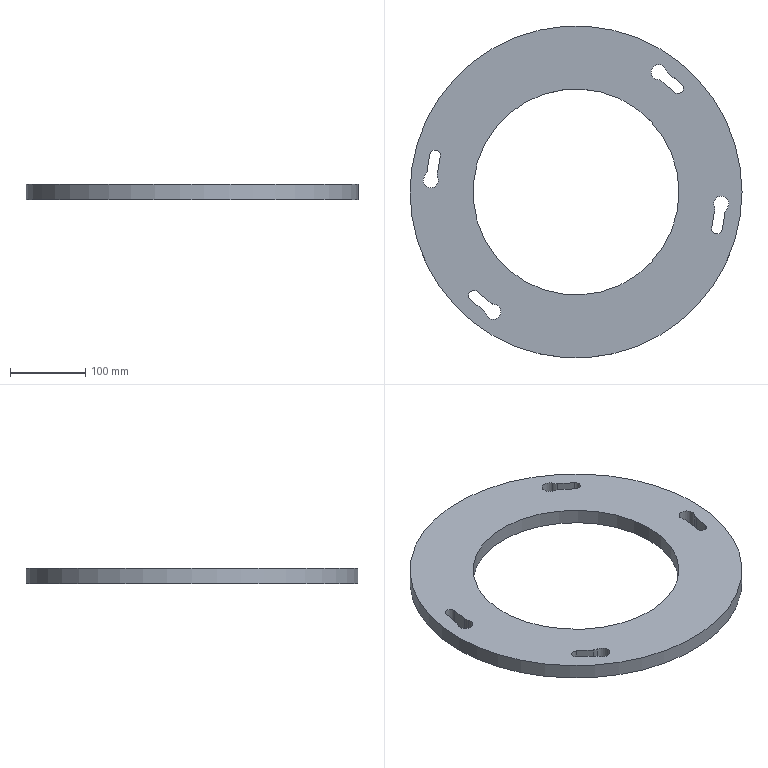NC program | NX | posted with a generic post | part box 440 x 440 x 20 mm
Lines 1 to 784 of 7039:
N10 G17 G21 G94 G90
(ZLEVEL_PROFILE_COPY_1 , TOOL : D10)
N12 T10 M6
N14 G54
N16 G17 G0 G90 X-122.22 Y-146.019 S2200 M3
N18 G43 Z80. H10
N20 Z1.5
N22 G94 G1 X-134.503 Y-135.858 Z0.665 F2200.
N24 X-134.722 Y-135.75 Z0.652
N26 X-135.025 Y-135.606 Z0.634
N28 X-135.519 Y-135.541 Z0.608
N30 X-136.012 Y-135.608 Z0.582
N32 X-136.314 Y-135.752 Z0.564
N34 Y-135.831 Z0.56
N36 X-136.345 Y-135.857 Z0.558
N38 X-136.423 Y-135.84 Z0.554
N40 X-136.449 Y-135.824 Z0.552
N42 X-136.738 Y-135.992 Z0.535
N44 X-137.073 Y-136.368 Z0.509
N46 X-137.215 Y-136.689 Z0.49
N48 X-137.347 Y-136.996 Z0.473
N50 X-137.354 Y-137.814 Z0.43
N52 X-137.214 Y-138.155 Z0.41
N54 X-137.081 Y-138.462 Z0.393
N56 X-136.953 Y-138.633 Z0.382
N58 X-128.11 Y-145.949 Z-0.22
N60 X-119.524 Y-153.051
N62 G2 X-114.128 Y-160.588 R18.15
N64 G3 X-112.621 Y-162.654 R4.85
N66 G1 X-112.486 Y-162.758
N68 G3 X-106.443 Y-162.552 R4.85
N70 G1 X-105.654 Y-161.694
N72 G3 X-104.895 Y-160.066 R4.85
N74 G1 X-104.918 Y-160.045
N76 X-104.885 Y-160.028
N78 G3 X-104.883 Y-157.71 R4.85
N80 G1 X-104.918 Y-157.689
N82 X-104.893 Y-157.672
N84 G3 X-105.845 Y-155.789 R4.85
N86 G1 X-106.646 Y-155.014
N88 G3 X-108.751 Y-154.089 R4.85
N90 G2 X-117.166 Y-150.2 R18.15
N92 G1 X-134.336 Y-135.996
N94 G3 X-136.314 Y-135.752 R1.85
N96 G1 X-136.305 Y-135.819
N98 X-136.359 Y-135.863
N100 X-136.423 Y-135.84
N102 X-136.449 Y-135.824
N104 G3 X-136.695 Y-138.846 R1.85
N106 G1 X-128.11 Y-145.949
N108 X-119.549 Y-153.03 Z-0.414
N110 X-119.266 Y-153.269 Z-0.42
N112 X-118.988 Y-153.513 Z-0.427
N114 X-118.714 Y-153.763 Z-0.433
N116 X-118.446 Y-154.018 Z-0.44
N118 G2 X-114.128 Y-160.588 R18.15
N120 G3 X-112.621 Y-162.654 R4.85
N122 G1 X-112.486 Y-162.758
N124 G3 X-106.443 Y-162.552 R4.85
N126 G1 X-105.654 Y-161.694
N128 G3 X-104.895 Y-160.066 R4.85
N130 G1 X-104.918 Y-160.045
N132 X-104.885 Y-160.028
N134 G3 X-104.883 Y-157.71 R4.85
N136 G1 X-104.918 Y-157.689
N138 X-104.893 Y-157.672
N140 G3 X-105.845 Y-155.789 R4.85
N142 G1 X-106.646 Y-155.014
N144 G3 X-108.751 Y-154.089 R4.85
N146 G2 X-117.166 Y-150.2 R18.15
N148 G1 X-134.336 Y-135.996
N150 G3 X-136.314 Y-135.752 R1.85
N152 G1 X-136.305 Y-135.819
N154 X-136.359 Y-135.863
N156 X-136.423 Y-135.84
N158 X-136.449 Y-135.824
N160 G3 X-136.695 Y-138.846 R1.85
N162 G1 X-128.11 Y-145.949
N164 X-119.549 Y-153.03 Z-0.633
N166 X-119.266 Y-153.269 Z-0.64
N168 X-118.988 Y-153.513 Z-0.646
N170 X-118.714 Y-153.763 Z-0.653
N172 X-118.446 Y-154.018 Z-0.659
N174 G2 X-114.128 Y-160.588 R18.15
N176 G3 X-112.621 Y-162.654 R4.85
N178 G1 X-112.486 Y-162.758
N180 G3 X-106.443 Y-162.552 R4.85
N182 G1 X-105.654 Y-161.694
N184 G3 X-104.895 Y-160.066 R4.85
N186 G1 X-104.918 Y-160.045
N188 X-104.885 Y-160.028
N190 G3 X-104.883 Y-157.71 R4.85
N192 G1 X-104.918 Y-157.689
N194 X-104.893 Y-157.672
N196 G3 X-105.845 Y-155.789 R4.85
N198 G1 X-106.646 Y-155.014
N200 G3 X-108.751 Y-154.089 R4.85
N202 G2 X-117.166 Y-150.2 R18.15
N204 G1 X-134.336 Y-135.996
N206 G3 X-136.314 Y-135.752 R1.85
N208 G1 X-136.305 Y-135.819
N210 X-136.359 Y-135.863
N212 X-136.423 Y-135.84
N214 X-136.449 Y-135.824
N216 G3 X-136.695 Y-138.846 R1.85
N218 G1 X-128.11 Y-145.949
N220 X-119.549 Y-153.03 Z-0.853
N222 X-119.266 Y-153.269 Z-0.86
N224 X-118.988 Y-153.513 Z-0.866
N226 X-118.714 Y-153.763 Z-0.873
N228 X-118.446 Y-154.018 Z-0.879
N230 G2 X-114.128 Y-160.588 R18.15
N232 G3 X-112.621 Y-162.654 R4.85
N234 G1 X-112.486 Y-162.758
N236 G3 X-106.443 Y-162.552 R4.85
N238 G1 X-105.654 Y-161.694
N240 G3 X-104.895 Y-160.066 R4.85
N242 G1 X-104.918 Y-160.045
N244 X-104.885 Y-160.028
N246 G3 X-104.883 Y-157.71 R4.85
N248 G1 X-104.918 Y-157.689
N250 X-104.893 Y-157.672
N252 G3 X-105.845 Y-155.789 R4.85
N254 G1 X-106.646 Y-155.014
N256 G3 X-108.751 Y-154.089 R4.85
N258 G2 X-117.166 Y-150.2 R18.15
N260 G1 X-134.336 Y-135.996
N262 G3 X-136.314 Y-135.752 R1.85
N264 G1 X-136.305 Y-135.819
N266 X-136.359 Y-135.863
N268 X-136.423 Y-135.84
N270 X-136.449 Y-135.824
N272 G3 X-136.695 Y-138.846 R1.85
N274 G1 X-128.11 Y-145.949
N276 X-119.549 Y-153.03 Z-1.073
N278 X-119.266 Y-153.269 Z-1.08
N280 X-118.988 Y-153.513 Z-1.086
N282 X-118.714 Y-153.763 Z-1.092
N284 X-118.446 Y-154.018 Z-1.099
N286 G2 X-114.128 Y-160.588 R18.15
N288 G3 X-112.621 Y-162.654 R4.85
N290 G1 X-112.486 Y-162.758
N292 G3 X-106.443 Y-162.552 R4.85
N294 G1 X-105.654 Y-161.694
N296 G3 X-104.895 Y-160.066 R4.85
N298 G1 X-104.918 Y-160.045
N300 X-104.885 Y-160.028
N302 G3 X-104.883 Y-157.71 R4.85
N304 G1 X-104.918 Y-157.689
N306 X-104.893 Y-157.672
N308 G3 X-105.845 Y-155.789 R4.85
N310 G1 X-106.646 Y-155.014
N312 G3 X-108.751 Y-154.089 R4.85
N314 G2 X-117.166 Y-150.2 R18.15
N316 G1 X-134.336 Y-135.996
N318 G3 X-136.314 Y-135.752 R1.85
N320 G1 X-136.305 Y-135.819
N322 X-136.359 Y-135.863
N324 X-136.423 Y-135.84
N326 X-136.449 Y-135.824
N328 G3 X-136.695 Y-138.846 R1.85
N330 G1 X-128.11 Y-145.949
N332 X-119.549 Y-153.03 Z-1.293
N334 X-119.266 Y-153.269 Z-1.299
N336 X-118.988 Y-153.513 Z-1.306
N338 X-118.714 Y-153.763 Z-1.312
N340 X-118.446 Y-154.018 Z-1.319
N342 G2 X-114.128 Y-160.588 R18.15
N344 G3 X-112.621 Y-162.654 R4.85
N346 G1 X-112.486 Y-162.758
N348 G3 X-106.443 Y-162.552 R4.85
N350 G1 X-105.654 Y-161.694
N352 G3 X-104.895 Y-160.066 R4.85
N354 G1 X-104.918 Y-160.045
N356 X-104.885 Y-160.028
N358 G3 X-104.883 Y-157.71 R4.85
N360 G1 X-104.918 Y-157.689
N362 X-104.893 Y-157.672
N364 G3 X-105.845 Y-155.789 R4.85
N366 G1 X-106.646 Y-155.014
N368 G3 X-108.751 Y-154.089 R4.85
N370 G2 X-117.166 Y-150.2 R18.15
N372 G1 X-134.336 Y-135.996
N374 G3 X-136.314 Y-135.752 R1.85
N376 G1 X-136.305 Y-135.819
N378 X-136.359 Y-135.863
N380 X-136.423 Y-135.84
N382 X-136.449 Y-135.824
N384 G3 X-136.695 Y-138.846 R1.85
N386 G1 X-128.11 Y-145.949
N388 X-119.549 Y-153.03 Z-1.513
N390 X-119.266 Y-153.269 Z-1.519
N392 X-118.988 Y-153.513 Z-1.526
N394 X-118.714 Y-153.763 Z-1.532
N396 X-118.446 Y-154.018 Z-1.538
N398 G2 X-114.128 Y-160.588 R18.15
N400 G3 X-112.621 Y-162.654 R4.85
N402 G1 X-112.486 Y-162.758
N404 G3 X-106.443 Y-162.552 R4.85
N406 G1 X-105.654 Y-161.694
N408 G3 X-104.895 Y-160.066 R4.85
N410 G1 X-104.918 Y-160.045
N412 X-104.885 Y-160.028
N414 G3 X-104.883 Y-157.71 R4.85
N416 G1 X-104.918 Y-157.689
N418 X-104.893 Y-157.672
N420 G3 X-105.845 Y-155.789 R4.85
N422 G1 X-106.646 Y-155.014
N424 G3 X-108.751 Y-154.089 R4.85
N426 G2 X-117.166 Y-150.2 R18.15
N428 G1 X-134.336 Y-135.996
N430 G3 X-136.314 Y-135.752 R1.85
N432 G1 X-136.305 Y-135.819
N434 X-136.359 Y-135.863
N436 X-136.423 Y-135.84
N438 X-136.449 Y-135.824
N440 G3 X-136.695 Y-138.846 R1.85
N442 G1 X-128.11 Y-145.949
N444 X-119.549 Y-153.03 Z-1.732
N446 X-119.266 Y-153.269 Z-1.739
N448 X-118.988 Y-153.513 Z-1.745
N450 X-118.714 Y-153.763 Z-1.752
N452 X-118.446 Y-154.018 Z-1.758
N454 G2 X-114.128 Y-160.588 R18.15
N456 G3 X-112.621 Y-162.654 R4.85
N458 G1 X-112.486 Y-162.758
N460 G3 X-106.443 Y-162.552 R4.85
N462 G1 X-105.654 Y-161.694
N464 G3 X-104.895 Y-160.066 R4.85
N466 G1 X-104.918 Y-160.045
N468 X-104.885 Y-160.028
N470 G3 X-104.883 Y-157.71 R4.85
N472 G1 X-104.918 Y-157.689
N474 X-104.893 Y-157.672
N476 G3 X-105.845 Y-155.789 R4.85
N478 G1 X-106.646 Y-155.014
N480 G3 X-108.751 Y-154.089 R4.85
N482 G2 X-117.166 Y-150.2 R18.15
N484 G1 X-134.336 Y-135.996
N486 G3 X-136.314 Y-135.752 R1.85
N488 G1 X-136.305 Y-135.819
N490 X-136.359 Y-135.863
N492 X-136.423 Y-135.84
N494 X-136.449 Y-135.824
N496 G3 X-136.695 Y-138.846 R1.85
N498 G1 X-128.11 Y-145.949
N500 X-119.549 Y-153.03 Z-1.952
N502 X-119.266 Y-153.269 Z-1.959
N504 X-118.988 Y-153.513 Z-1.965
N506 X-118.714 Y-153.763 Z-1.972
N508 X-118.446 Y-154.018 Z-1.978
N510 G2 X-114.128 Y-160.588 R18.15
N512 G3 X-112.621 Y-162.654 R4.85
N514 G1 X-112.486 Y-162.758
N516 G3 X-106.443 Y-162.552 R4.85
N518 G1 X-105.654 Y-161.694
N520 G3 X-104.895 Y-160.066 R4.85
N522 G1 X-104.918 Y-160.045
N524 X-104.885 Y-160.028
N526 G3 X-104.883 Y-157.71 R4.85
N528 G1 X-104.918 Y-157.689
N530 X-104.893 Y-157.672
N532 G3 X-105.845 Y-155.789 R4.85
N534 G1 X-106.646 Y-155.014
N536 G3 X-108.751 Y-154.089 R4.85
N538 G2 X-117.166 Y-150.2 R18.15
N540 G1 X-134.336 Y-135.996
N542 G3 X-136.314 Y-135.752 R1.85
N544 G1 X-136.305 Y-135.819
N546 X-136.359 Y-135.863
N548 X-136.423 Y-135.84
N550 X-136.449 Y-135.824
N552 G3 X-136.695 Y-138.846 R1.85
N554 G1 X-128.11 Y-145.949
N556 X-119.549 Y-153.03 Z-2.172
N558 X-119.266 Y-153.269 Z-2.178
N560 X-118.988 Y-153.513 Z-2.185
N562 X-118.714 Y-153.763 Z-2.191
N564 X-118.446 Y-154.018 Z-2.198
N566 G2 X-114.128 Y-160.588 R18.15
N568 G3 X-112.621 Y-162.654 R4.85
N570 G1 X-112.486 Y-162.758
N572 G3 X-106.443 Y-162.552 R4.85
N574 G1 X-105.654 Y-161.694
N576 G3 X-104.895 Y-160.066 R4.85
N578 G1 X-104.918 Y-160.045
N580 X-104.885 Y-160.028
N582 G3 X-104.883 Y-157.71 R4.85
N584 G1 X-104.918 Y-157.689
N586 X-104.893 Y-157.672
N588 G3 X-105.845 Y-155.789 R4.85
N590 G1 X-106.646 Y-155.014
N592 G3 X-108.751 Y-154.089 R4.85
N594 G2 X-117.166 Y-150.2 R18.15
N596 G1 X-134.336 Y-135.996
N598 G3 X-136.314 Y-135.752 R1.85
N600 G1 X-136.305 Y-135.819
N602 X-136.359 Y-135.863
N604 X-136.423 Y-135.84
N606 X-136.449 Y-135.824
N608 G3 X-136.695 Y-138.846 R1.85
N610 G1 X-128.11 Y-145.949
N612 X-119.549 Y-153.03 Z-2.392
N614 X-119.266 Y-153.269 Z-2.398
N616 X-118.988 Y-153.513 Z-2.405
N618 X-118.714 Y-153.763 Z-2.411
N620 X-118.446 Y-154.018 Z-2.418
N622 G2 X-114.128 Y-160.588 R18.15
N624 G3 X-112.621 Y-162.654 R4.85
N626 G1 X-112.486 Y-162.758
N628 G3 X-106.443 Y-162.552 R4.85
N630 G1 X-105.654 Y-161.694
N632 G3 X-104.895 Y-160.066 R4.85
N634 G1 X-104.918 Y-160.045
N636 X-104.885 Y-160.028
N638 G3 X-104.883 Y-157.71 R4.85
N640 G1 X-104.918 Y-157.689
N642 X-104.893 Y-157.672
N644 G3 X-105.845 Y-155.789 R4.85
N646 G1 X-106.646 Y-155.014
N648 G3 X-108.751 Y-154.089 R4.85
N650 G2 X-117.166 Y-150.2 R18.15
N652 G1 X-134.336 Y-135.996
N654 G3 X-136.314 Y-135.752 R1.85
N656 G1 X-136.305 Y-135.819
N658 X-136.359 Y-135.863
N660 X-136.423 Y-135.84
N662 X-136.449 Y-135.824
N664 G3 X-136.695 Y-138.846 R1.85
N666 G1 X-128.11 Y-145.949
N668 X-119.549 Y-153.03 Z-2.612
N670 X-119.266 Y-153.269 Z-2.618
N672 X-118.988 Y-153.513 Z-2.624
N674 X-118.714 Y-153.763 Z-2.631
N676 X-118.446 Y-154.018 Z-2.637
N678 G2 X-114.128 Y-160.588 R18.15
N680 G3 X-112.621 Y-162.654 R4.85
N682 G1 X-112.486 Y-162.758
N684 G3 X-106.443 Y-162.552 R4.85
N686 G1 X-105.654 Y-161.694
N688 G3 X-104.895 Y-160.066 R4.85
N690 G1 X-104.918 Y-160.045
N692 X-104.885 Y-160.028
N694 G3 X-104.883 Y-157.71 R4.85
N696 G1 X-104.918 Y-157.689
N698 X-104.893 Y-157.672
N700 G3 X-105.845 Y-155.789 R4.85
N702 G1 X-106.646 Y-155.014
N704 G3 X-108.751 Y-154.089 R4.85
N706 G2 X-117.166 Y-150.2 R18.15
N708 G1 X-134.336 Y-135.996
N710 G3 X-136.314 Y-135.752 R1.85
N712 G1 X-136.305 Y-135.819
N714 X-136.359 Y-135.863
N716 X-136.423 Y-135.84
N718 X-136.449 Y-135.824
N720 G3 X-136.695 Y-138.846 R1.85
N722 G1 X-128.11 Y-145.949
N724 X-119.549 Y-153.03 Z-2.831
N726 X-119.266 Y-153.269 Z-2.838
N728 X-118.988 Y-153.513 Z-2.844
N730 X-118.714 Y-153.763 Z-2.851
N732 X-118.446 Y-154.018 Z-2.857
N734 G2 X-114.128 Y-160.588 R18.15
N736 G3 X-112.621 Y-162.654 R4.85
N738 G1 X-112.486 Y-162.758
N740 G3 X-106.443 Y-162.552 R4.85
N742 G1 X-105.654 Y-161.694
N744 G3 X-104.895 Y-160.066 R4.85
N746 G1 X-104.918 Y-160.045
N748 X-104.885 Y-160.028
N750 G3 X-104.883 Y-157.71 R4.85
N752 G1 X-104.918 Y-157.689
N754 X-104.893 Y-157.672
N756 G3 X-105.845 Y-155.789 R4.85
N758 G1 X-106.646 Y-155.014
N760 G3 X-108.751 Y-154.089 R4.85
N762 G2 X-117.166 Y-150.2 R18.15
N764 G1 X-134.336 Y-135.996
N766 G3 X-136.314 Y-135.752 R1.85
N768 G1 X-136.305 Y-135.819
N770 X-136.359 Y-135.863
N772 X-136.423 Y-135.84
N774 X-136.449 Y-135.824
N776 G3 X-136.695 Y-138.846 R1.85
N778 G1 X-128.11 Y-145.949
N780 X-119.549 Y-153.03 Z-3.051
N782 X-119.266 Y-153.269 Z-3.058
N784 X-118.988 Y-153.513 Z-3.064
N786 X-118.714 Y-153.763 Z-3.07
N788 X-118.446 Y-154.018 Z-3.077
N790 G2 X-114.128 Y-160.588 R18.15
N792 G3 X-112.621 Y-162.654 R4.85
N794 G1 X-112.486 Y-162.758
N796 G3 X-106.443 Y-162.552 R4.85
N798 G1 X-105.654 Y-161.694
N800 G3 X-104.895 Y-160.066 R4.85
N802 G1 X-104.918 Y-160.045
N804 X-104.885 Y-160.028
N806 G3 X-104.883 Y-157.71 R4.85
N808 G1 X-104.918 Y-157.689
N810 X-104.893 Y-157.672
N812 G3 X-105.845 Y-155.789 R4.85
N814 G1 X-106.646 Y-155.014
N816 G3 X-108.751 Y-154.089 R4.85
N818 G2 X-117.166 Y-150.2 R18.15
N820 G1 X-134.336 Y-135.996
N822 G3 X-136.314 Y-135.752 R1.85
N824 G1 X-136.305 Y-135.819
N826 X-136.359 Y-135.863
N828 X-136.423 Y-135.84
N830 X-136.449 Y-135.824
N832 G3 X-136.695 Y-138.846 R1.85
N834 G1 X-128.11 Y-145.949
N836 X-119.549 Y-153.03 Z-3.271
N838 X-119.266 Y-153.269 Z-3.277
N840 X-118.988 Y-153.513 Z-3.284
N842 X-118.714 Y-153.763 Z-3.29
N844 X-118.446 Y-154.018 Z-3.297
N846 G2 X-114.128 Y-160.588 R18.15
N848 G3 X-112.621 Y-162.654 R4.85
N850 G1 X-112.486 Y-162.758
N852 G3 X-106.443 Y-162.552 R4.85
N854 G1 X-105.654 Y-161.694
N856 G3 X-104.895 Y-160.066 R4.85
N858 G1 X-104.918 Y-160.045
N860 X-104.885 Y-160.028
N862 G3 X-104.883 Y-157.71 R4.85
N864 G1 X-104.918 Y-157.689
N866 X-104.893 Y-157.672
N868 G3 X-105.845 Y-155.789 R4.85
N870 G1 X-106.646 Y-155.014
N872 G3 X-108.751 Y-154.089 R4.85
N874 G2 X-117.166 Y-150.2 R18.15
N876 G1 X-134.336 Y-135.996
N878 G3 X-136.314 Y-135.752 R1.85
N880 G1 X-136.305 Y-135.819
N882 X-136.359 Y-135.863
N884 X-136.423 Y-135.84
N886 X-136.449 Y-135.824
N888 G3 X-136.695 Y-138.846 R1.85
N890 G1 X-128.11 Y-145.949
N892 X-119.549 Y-153.03 Z-3.491
N894 X-119.266 Y-153.269 Z-3.497
N896 X-118.988 Y-153.513 Z-3.504
N898 X-118.714 Y-153.763 Z-3.51
N900 X-118.446 Y-154.018 Z-3.516
N902 G2 X-114.128 Y-160.588 R18.15
N904 G3 X-112.621 Y-162.654 R4.85
N906 G1 X-112.486 Y-162.758
N908 G3 X-106.443 Y-162.552 R4.85
N910 G1 X-105.654 Y-161.694
N912 G3 X-104.895 Y-160.066 R4.85
N914 G1 X-104.918 Y-160.045
N916 X-104.885 Y-160.028
N918 G3 X-104.883 Y-157.71 R4.85
N920 G1 X-104.918 Y-157.689
N922 X-104.893 Y-157.672
N924 G3 X-105.845 Y-155.789 R4.85
N926 G1 X-106.646 Y-155.014
N928 G3 X-108.751 Y-154.089 R4.85
N930 G2 X-117.166 Y-150.2 R18.15
N932 G1 X-134.336 Y-135.996
N934 G3 X-136.314 Y-135.752 R1.85
N936 G1 X-136.305 Y-135.819
N938 X-136.359 Y-135.863
N940 X-136.423 Y-135.84
N942 X-136.449 Y-135.824
N944 G3 X-136.695 Y-138.846 R1.85
N946 G1 X-128.11 Y-145.949
N948 X-119.549 Y-153.03 Z-3.71
N950 X-119.266 Y-153.269 Z-3.717
N952 X-118.988 Y-153.513 Z-3.723
N954 X-118.714 Y-153.763 Z-3.73
N956 X-118.446 Y-154.018 Z-3.736
N958 G2 X-114.128 Y-160.588 R18.15
N960 G3 X-112.621 Y-162.654 R4.85
N962 G1 X-112.486 Y-162.758
N964 G3 X-106.443 Y-162.552 R4.85
N966 G1 X-105.654 Y-161.694
N968 G3 X-104.895 Y-160.066 R4.85
N970 G1 X-104.918 Y-160.045
N972 X-104.885 Y-160.028
N974 G3 X-104.883 Y-157.71 R4.85
N976 G1 X-104.918 Y-157.689
N978 X-104.893 Y-157.672
N980 G3 X-105.845 Y-155.789 R4.85
N982 G1 X-106.646 Y-155.014
N984 G3 X-108.751 Y-154.089 R4.85
N986 G2 X-117.166 Y-150.2 R18.15
N988 G1 X-134.336 Y-135.996
N990 G3 X-136.314 Y-135.752 R1.85
N992 G1 X-136.305 Y-135.819
N994 X-136.359 Y-135.863
N996 X-136.423 Y-135.84
N998 X-136.449 Y-135.824
N1000 G3 X-136.695 Y-138.846 R1.85
N1002 G1 X-128.11 Y-145.949
N1004 X-119.549 Y-153.03 Z-3.93
N1006 X-119.266 Y-153.269 Z-3.937
N1008 X-118.988 Y-153.513 Z-3.943
N1010 X-118.714 Y-153.763 Z-3.95
N1012 X-118.446 Y-154.018 Z-3.956
N1014 G2 X-114.128 Y-160.588 R18.15
N1016 G3 X-112.621 Y-162.654 R4.85
N1018 G1 X-112.486 Y-162.758
N1020 G3 X-106.443 Y-162.552 R4.85
N1022 G1 X-105.654 Y-161.694
N1024 G3 X-104.895 Y-160.066 R4.85
N1026 G1 X-104.918 Y-160.045
N1028 X-104.885 Y-160.028
N1030 G3 X-104.883 Y-157.71 R4.85
N1032 G1 X-104.918 Y-157.689
N1034 X-104.893 Y-157.672
N1036 G3 X-105.845 Y-155.789 R4.85
N1038 G1 X-106.646 Y-155.014
N1040 G3 X-108.751 Y-154.089 R4.85
N1042 G2 X-117.166 Y-150.2 R18.15
N1044 G1 X-134.336 Y-135.996
N1046 G3 X-136.314 Y-135.752 R1.85
N1048 G1 X-136.305 Y-135.819
N1050 X-136.359 Y-135.863
N1052 X-136.423 Y-135.84
N1054 X-136.449 Y-135.824
N1056 G3 X-136.695 Y-138.846 R1.85
N1058 G1 X-128.11 Y-145.949
N1060 X-119.549 Y-153.03 Z-4.15
N1062 X-119.266 Y-153.269 Z-4.156
N1064 X-118.988 Y-153.513 Z-4.163
N1066 X-118.714 Y-153.763 Z-4.169
N1068 X-118.446 Y-154.018 Z-4.176
N1070 G2 X-114.128 Y-160.588 R18.15
N1072 G3 X-112.621 Y-162.654 R4.85
N1074 G1 X-112.486 Y-162.758
N1076 G3 X-106.443 Y-162.552 R4.85
N1078 G1 X-105.654 Y-161.694
N1080 G3 X-104.895 Y-160.066 R4.85
N1082 G1 X-104.918 Y-160.045
N1084 X-104.885 Y-160.028
N1086 G3 X-104.883 Y-157.71 R4.85
N1088 G1 X-104.918 Y-157.689
N1090 X-104.893 Y-157.672
N1092 G3 X-105.845 Y-155.789 R4.85
N1094 G1 X-106.646 Y-155.014
N1096 G3 X-108.751 Y-154.089 R4.85
N1098 G2 X-117.166 Y-150.2 R18.15
N1100 G1 X-134.336 Y-135.996
N1102 G3 X-136.314 Y-135.752 R1.85
N1104 G1 X-136.305 Y-135.819
N1106 X-136.359 Y-135.863
N1108 X-136.423 Y-135.84
N1110 X-136.449 Y-135.824
N1112 G3 X-136.695 Y-138.846 R1.85
N1114 G1 X-128.11 Y-145.949
N1116 X-119.549 Y-153.03 Z-4.37
N1118 X-119.266 Y-153.269 Z-4.376
N1120 X-118.988 Y-153.513 Z-4.383
N1122 X-118.714 Y-153.763 Z-4.389
N1124 X-118.446 Y-154.018 Z-4.396
N1126 G2 X-114.128 Y-160.588 R18.15
N1128 G3 X-112.621 Y-162.654 R4.85
N1130 G1 X-112.486 Y-162.758
N1132 G3 X-106.443 Y-162.552 R4.85
N1134 G1 X-105.654 Y-161.694
N1136 G3 X-104.895 Y-160.066 R4.85
N1138 G1 X-104.918 Y-160.045
N1140 X-104.885 Y-160.028
N1142 G3 X-104.883 Y-157.71 R4.85
N1144 G1 X-104.918 Y-157.689
N1146 X-104.893 Y-157.672
N1148 G3 X-105.845 Y-155.789 R4.85
N1150 G1 X-106.646 Y-155.014
N1152 G3 X-108.751 Y-154.089 R4.85
N1154 G2 X-117.166 Y-150.2 R18.15
N1156 G1 X-134.336 Y-135.996
N1158 G3 X-136.314 Y-135.752 R1.85
N1160 G1 X-136.305 Y-135.819
N1162 X-136.359 Y-135.863
N1164 X-136.423 Y-135.84
N1166 X-136.449 Y-135.824
N1168 G3 X-136.695 Y-138.846 R1.85
N1170 G1 X-128.11 Y-145.949
N1172 X-119.549 Y-153.03 Z-4.59
N1174 X-119.266 Y-153.269 Z-4.596
N1176 X-118.988 Y-153.513 Z-4.602
N1178 X-118.714 Y-153.763 Z-4.609
N1180 X-118.446 Y-154.018 Z-4.615
N1182 G2 X-114.128 Y-160.588 R18.15
N1184 G3 X-112.621 Y-162.654 R4.85
N1186 G1 X-112.486 Y-162.758
N1188 G3 X-106.443 Y-162.552 R4.85
N1190 G1 X-105.654 Y-161.694
N1192 G3 X-104.895 Y-160.066 R4.85
N1194 G1 X-104.918 Y-160.045
N1196 X-104.885 Y-160.028
N1198 G3 X-104.883 Y-157.71 R4.85
N1200 G1 X-104.918 Y-157.689
N1202 X-104.893 Y-157.672
N1204 G3 X-105.845 Y-155.789 R4.85
N1206 G1 X-106.646 Y-155.014
N1208 G3 X-108.751 Y-154.089 R4.85
N1210 G2 X-117.166 Y-150.2 R18.15
N1212 G1 X-134.336 Y-135.996
N1214 G3 X-136.314 Y-135.752 R1.85
N1216 G1 X-136.305 Y-135.819
N1218 X-136.359 Y-135.863
N1220 X-136.423 Y-135.84
N1222 X-136.449 Y-135.824
N1224 G3 X-136.695 Y-138.846 R1.85
N1226 G1 X-128.11 Y-145.949
N1228 X-119.549 Y-153.03 Z-4.809
N1230 X-119.266 Y-153.269 Z-4.816
N1232 X-118.988 Y-153.513 Z-4.822
N1234 X-118.714 Y-153.763 Z-4.829
N1236 X-118.446 Y-154.018 Z-4.835
N1238 G2 X-114.128 Y-160.588 R18.15
N1240 G3 X-112.621 Y-162.654 R4.85
N1242 G1 X-112.486 Y-162.758
N1244 G3 X-106.443 Y-162.552 R4.85
N1246 G1 X-105.654 Y-161.694
N1248 G3 X-104.895 Y-160.066 R4.85
N1250 G1 X-104.918 Y-160.045
N1252 X-104.885 Y-160.028
N1254 G3 X-104.883 Y-157.71 R4.85
N1256 G1 X-104.918 Y-157.689
N1258 X-104.893 Y-157.672
N1260 G3 X-105.845 Y-155.789 R4.85
N1262 G1 X-106.646 Y-155.014
N1264 G3 X-108.751 Y-154.089 R4.85
N1266 G2 X-117.166 Y-150.2 R18.15
N1268 G1 X-134.336 Y-135.996
N1270 G3 X-136.314 Y-135.752 R1.85
N1272 G1 X-136.305 Y-135.819
N1274 X-136.359 Y-135.863
N1276 X-136.423 Y-135.84
N1278 X-136.449 Y-135.824
N1280 G3 X-136.695 Y-138.846 R1.85
N1282 G1 X-128.11 Y-145.949
N1284 X-119.549 Y-153.03 Z-5.029
N1286 X-119.266 Y-153.269 Z-5.036
N1288 X-118.988 Y-153.513 Z-5.042
N1290 X-118.714 Y-153.763 Z-5.048
N1292 X-118.446 Y-154.018 Z-5.055
N1294 G2 X-114.128 Y-160.588 R18.15
N1296 G3 X-112.621 Y-162.654 R4.85
N1298 G1 X-112.486 Y-162.758
N1300 G3 X-106.443 Y-162.552 R4.85
N1302 G1 X-105.654 Y-161.694
N1304 G3 X-104.895 Y-160.066 R4.85
N1306 G1 X-104.918 Y-160.045
N1308 X-104.885 Y-160.028
N1310 G3 X-104.883 Y-157.71 R4.85
N1312 G1 X-104.918 Y-157.689
N1314 X-104.893 Y-157.672
N1316 G3 X-105.845 Y-155.789 R4.85
N1318 G1 X-106.646 Y-155.014
N1320 G3 X-108.751 Y-154.089 R4.85
N1322 G2 X-117.166 Y-150.2 R18.15
N1324 G1 X-134.336 Y-135.996
N1326 G3 X-136.314 Y-135.752 R1.85
N1328 G1 X-136.305 Y-135.819
N1330 X-136.359 Y-135.863
N1332 X-136.423 Y-135.84
N1334 X-136.449 Y-135.824
N1336 G3 X-136.695 Y-138.846 R1.85
N1338 G1 X-128.11 Y-145.949
N1340 X-119.549 Y-153.03 Z-5.249
N1342 X-119.266 Y-153.269 Z-5.255
N1344 X-118.988 Y-153.513 Z-5.262
N1346 X-118.714 Y-153.763 Z-5.268
N1348 X-118.446 Y-154.018 Z-5.275
N1350 G2 X-114.128 Y-160.588 R18.15
N1352 G3 X-112.621 Y-162.654 R4.85
N1354 G1 X-112.486 Y-162.758
N1356 G3 X-106.443 Y-162.552 R4.85
N1358 G1 X-105.654 Y-161.694
N1360 G3 X-104.895 Y-160.066 R4.85
N1362 G1 X-104.918 Y-160.045
N1364 X-104.885 Y-160.028
N1366 G3 X-104.883 Y-157.71 R4.85
N1368 G1 X-104.918 Y-157.689
N1370 X-104.893 Y-157.672
N1372 G3 X-105.845 Y-155.789 R4.85
N1374 G1 X-106.646 Y-155.014
N1376 G3 X-108.751 Y-154.089 R4.85
N1378 G2 X-117.166 Y-150.2 R18.15
N1380 G1 X-134.336 Y-135.996
N1382 G3 X-136.314 Y-135.752 R1.85
N1384 G1 X-136.305 Y-135.819
N1386 X-136.359 Y-135.863
N1388 X-136.423 Y-135.84
N1390 X-136.449 Y-135.824
N1392 G3 X-136.695 Y-138.846 R1.85
N1394 G1 X-128.11 Y-145.949
N1396 X-119.549 Y-153.03 Z-5.469
N1398 X-119.266 Y-153.269 Z-5.475
N1400 X-118.988 Y-153.513 Z-5.482
N1402 X-118.714 Y-153.763 Z-5.488
N1404 X-118.446 Y-154.018 Z-5.495
N1406 G2 X-114.128 Y-160.588 R18.15
N1408 G3 X-112.621 Y-162.654 R4.85
N1410 G1 X-112.486 Y-162.758
N1412 G3 X-106.443 Y-162.552 R4.85
N1414 G1 X-105.654 Y-161.694
N1416 G3 X-104.895 Y-160.066 R4.85
N1418 G1 X-104.918 Y-160.045
N1420 X-104.885 Y-160.028
N1422 G3 X-104.883 Y-157.71 R4.85
N1424 G1 X-104.918 Y-157.689
N1426 X-104.893 Y-157.672
N1428 G3 X-105.845 Y-155.789 R4.85
N1430 G1 X-106.646 Y-155.014
N1432 G3 X-108.751 Y-154.089 R4.85
N1434 G2 X-117.166 Y-150.2 R18.15
N1436 G1 X-134.336 Y-135.996
N1438 G3 X-136.314 Y-135.752 R1.85
N1440 G1 X-136.305 Y-135.819
N1442 X-136.359 Y-135.863
N1444 X-136.423 Y-135.84
N1446 X-136.449 Y-135.824
N1448 G3 X-136.695 Y-138.846 R1.85
N1450 G1 X-128.11 Y-145.949
N1452 X-119.549 Y-153.03 Z-5.688
N1454 X-119.266 Y-153.269 Z-5.695
N1456 X-118.988 Y-153.513 Z-5.701
N1458 X-118.714 Y-153.763 Z-5.708
N1460 X-118.446 Y-154.018 Z-5.714
N1462 G2 X-114.128 Y-160.588 R18.15
N1464 G3 X-112.621 Y-162.654 R4.85
N1466 G1 X-112.486 Y-162.758
N1468 G3 X-106.443 Y-162.552 R4.85
N1470 G1 X-105.654 Y-161.694
N1472 G3 X-104.895 Y-160.066 R4.85
N1474 G1 X-104.918 Y-160.045
N1476 X-104.885 Y-160.028
N1478 G3 X-104.883 Y-157.71 R4.85
N1480 G1 X-104.918 Y-157.689
N1482 X-104.893 Y-157.672
N1484 G3 X-105.845 Y-155.789 R4.85
N1486 G1 X-106.646 Y-155.014
N1488 G3 X-108.751 Y-154.089 R4.85
N1490 G2 X-117.166 Y-150.2 R18.15
N1492 G1 X-134.336 Y-135.996
N1494 G3 X-136.314 Y-135.752 R1.85
N1496 G1 X-136.305 Y-135.819
N1498 X-136.359 Y-135.863
N1500 X-136.423 Y-135.84
N1502 X-136.449 Y-135.824
N1504 G3 X-136.695 Y-138.846 R1.85
N1506 G1 X-128.11 Y-145.949
N1508 X-119.549 Y-153.03 Z-5.908
N1510 X-119.266 Y-153.269 Z-5.915
N1512 X-118.988 Y-153.513 Z-5.921
N1514 X-118.714 Y-153.763 Z-5.928
N1516 X-118.446 Y-154.018 Z-5.934
N1518 G2 X-114.128 Y-160.588 R18.15
N1520 G3 X-112.621 Y-162.654 R4.85
N1522 G1 X-112.486 Y-162.758
N1524 G3 X-106.443 Y-162.552 R4.85
N1526 G1 X-105.654 Y-161.694
N1528 G3 X-104.895 Y-160.066 R4.85
N1530 G1 X-104.918 Y-160.045
N1532 X-104.885 Y-160.028
N1534 G3 X-104.883 Y-157.71 R4.85
N1536 G1 X-104.918 Y-157.689
N1538 X-104.893 Y-157.672
N1540 G3 X-105.845 Y-155.789 R4.85
N1542 G1 X-106.646 Y-155.014
N1544 G3 X-108.751 Y-154.089 R4.85
N1546 G2 X-117.166 Y-150.2 R18.15
N1548 G1 X-134.336 Y-135.996
N1550 G3 X-136.314 Y-135.752 R1.85
N1552 G1 X-136.305 Y-135.819
N1554 X-136.359 Y-135.863
N1556 X-136.423 Y-135.84
N1558 X-136.449 Y-135.824
N1560 G3 X-136.695 Y-138.846 R1.85
N1562 G1 X-128.11 Y-145.949
N1564 X-119.549 Y-153.03 Z-6.128
N1566 X-119.266 Y-153.269 Z-6.134